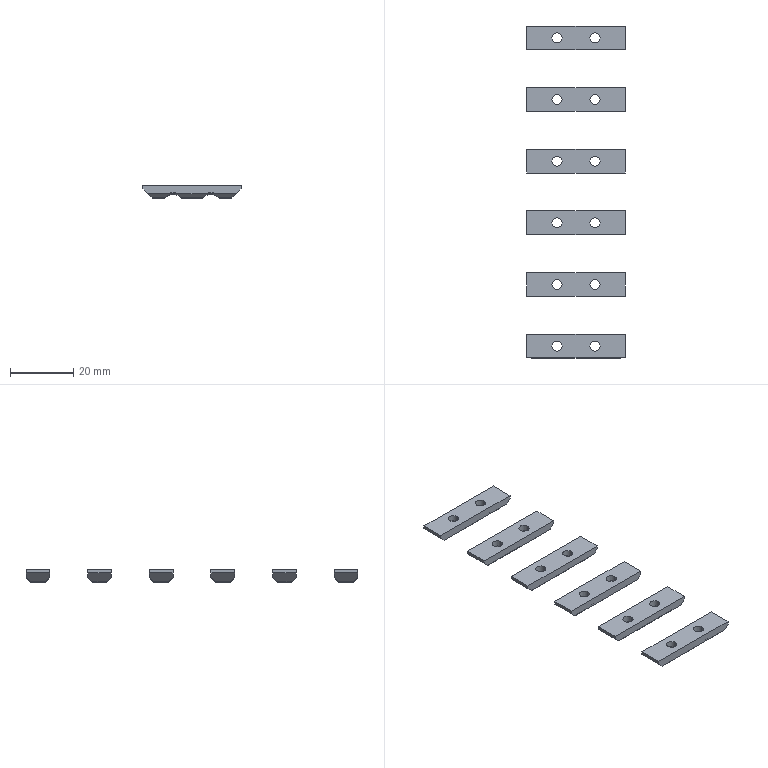Part | 6 solids | 600 faces | box 31 x 105 x 4 mm | volume 3740 mm3 | plane 306 | cylinder 294 | commonest cylinder face diameters 0.3 x246 3.2 x24 7 x24